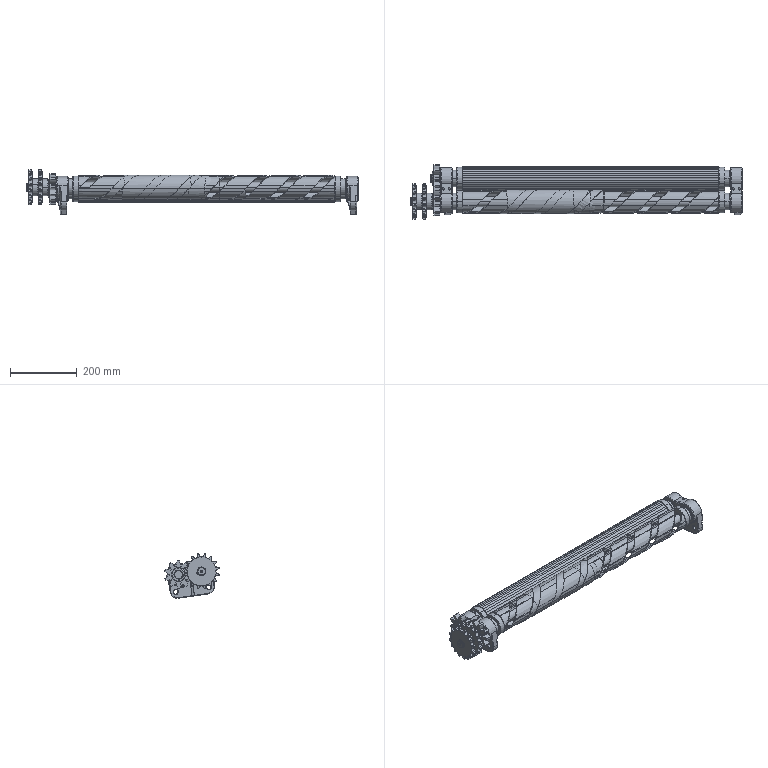Part | SolidWorks | features LayoutProfileFeature 1 | 27 solids | 1613 faces | box 994 x 163.102 x 133.781 mm | volume 7441719 mm3 | cylinder 762 | plane 382 | spline 327 | cone 142 | commonest cylinder face diameters 4 x74 19.857 x68 31.085 x64 70 x58 65 x48 76.673 x44